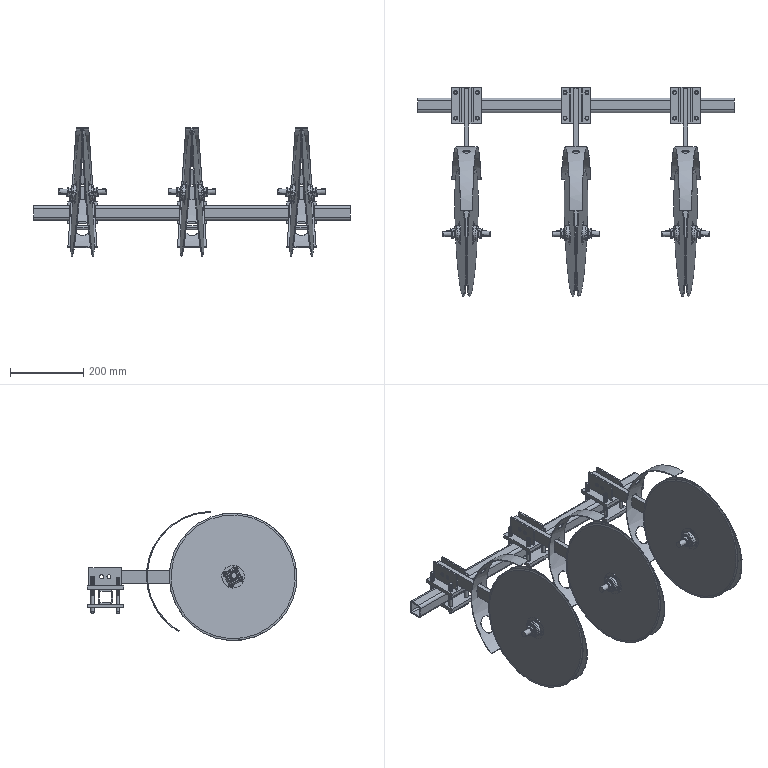Part | SolidWorks | features ReferencePattern 8, LocalLPattern 1 | 70 solids | 2283 faces | box 866 x 574.882 x 353.001 mm | volume 3236381 mm3 | cylinder 1511 | plane 412 | cone 108 | sphere 108 | torus 108 | spline 36 | commonest cylinder face diameters 10 x1032 4 x144 11 x84 31 x36 19 x27 15 x24